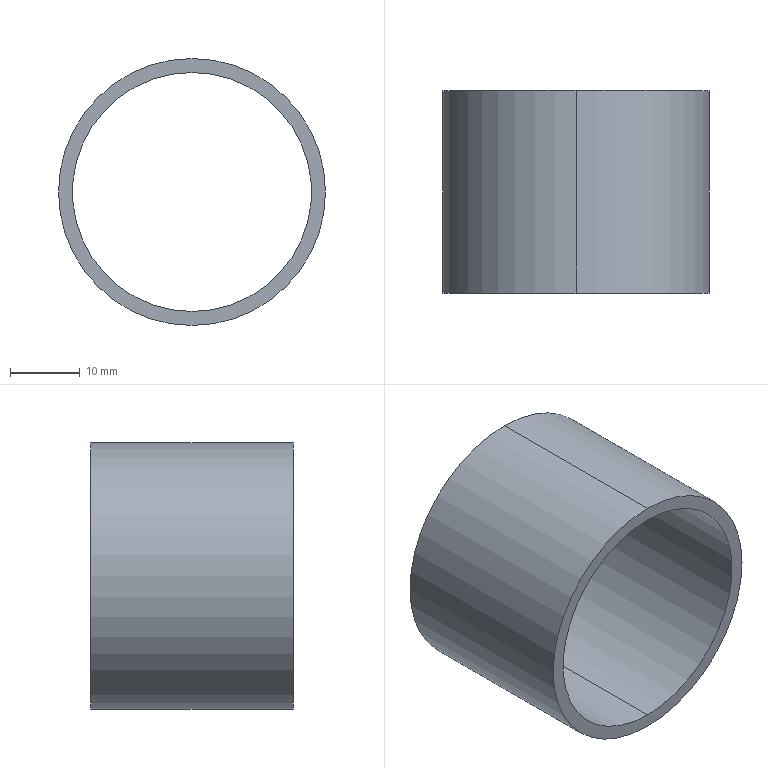Part | STEP file | Middle | 1 solid | 6 faces | box 38.2 x 29 x 38.2 mm | volume 6596 mm3 | cylinder 4 | plane 2 | commonest cylinder face diameters 34.2 x2 38.2 x2
STEP:
#1=CARTESIAN_POINT('',(0.,0.,0.));
#2=DIRECTION('',(0.,0.,1.));
#3=DIRECTION('',(1.,0.,0.));
#4=AXIS2_PLACEMENT_3D('',#1,#2,#3);
#5=CARTESIAN_POINT('',(0.,0.,17.1));
#6=VERTEX_POINT('',#5);
#7=CARTESIAN_POINT('',(0.,29.,17.1));
#8=VERTEX_POINT('',#7);
#9=CARTESIAN_POINT('',(0.,0.,17.1));
#10=DIRECTION('',(0.,1.,0.));
#11=VECTOR('',#10,1.);
#12=LINE('',#9,#11);
#13=CARTESIAN_POINT('',(0.,0.,0.));
#14=DIRECTION('',(0.,1.,0.));
#15=DIRECTION('',(0.,0.,1.));
#16=AXIS2_PLACEMENT_3D('',#13,#14,#15);
#17=CYLINDRICAL_SURFACE('',#16,17.1);
#18=CARTESIAN_POINT('',(6.283,0.));
#19=DIRECTION('',(0.,1.));
#20=VECTOR('',#19,1.);
#21=LINE('',#18,#20);
#22=(GEOMETRIC_REPRESENTATION_CONTEXT(2)PARAMETRIC_REPRESENTATION_CONTEXT()REPRESENTATION_CONTEXT('',''));
#23=DEFINITIONAL_REPRESENTATION('',(#21),#22);
#24=PCURVE('',#17,#23);
#25=CARTESIAN_POINT('',(0.,0.,0.));
#26=DIRECTION('',(0.,1.,0.));
#27=DIRECTION('',(0.,0.,1.));
#28=AXIS2_PLACEMENT_3D('',#25,#26,#27);
#29=CYLINDRICAL_SURFACE('',#28,17.1);
#30=CARTESIAN_POINT('',(0.,0.));
#31=DIRECTION('',(0.,1.));
#32=VECTOR('',#31,1.);
#33=LINE('',#30,#32);
#34=(GEOMETRIC_REPRESENTATION_CONTEXT(2)PARAMETRIC_REPRESENTATION_CONTEXT()REPRESENTATION_CONTEXT('',''));
#35=DEFINITIONAL_REPRESENTATION('',(#33),#34);
#36=PCURVE('',#29,#35);
#37=SURFACE_CURVE('',#12,(#24,#36),.PCURVE_S1.);
#38=EDGE_CURVE('',#6,#8,#37,.T.);
#39=ORIENTED_EDGE('',*,*,#38,.T.);
#40=CARTESIAN_POINT('',(0.,29.,-17.1));
#41=VERTEX_POINT('',#40);
#42=CARTESIAN_POINT('',(0.,29.,0.));
#43=DIRECTION('',(0.,1.,0.));
#44=DIRECTION('',(0.,0.,1.));
#45=AXIS2_PLACEMENT_3D('',#42,#43,#44);
#46=CIRCLE('',#45,17.1);
#47=CARTESIAN_POINT('',(0.,29.));
#48=DIRECTION('',(1.,0.));
#49=VECTOR('',#48,1.);
#50=LINE('',#47,#49);
#51=(GEOMETRIC_REPRESENTATION_CONTEXT(2)PARAMETRIC_REPRESENTATION_CONTEXT()REPRESENTATION_CONTEXT('',''));
#52=DEFINITIONAL_REPRESENTATION('',(#50),#51);
#53=PCURVE('',#17,#52);
#54=CARTESIAN_POINT('',(0.,29.,0.));
#55=DIRECTION('',(0.,1.,0.));
#56=DIRECTION('',(0.,0.,1.));
#57=AXIS2_PLACEMENT_3D('',#54,#55,#56);
#58=PLANE('',#57);
#59=CARTESIAN_POINT('',(0.,0.));
#60=DIRECTION('',(1.,0.));
#61=AXIS2_PLACEMENT_2D('',#59,#60);
#62=CIRCLE('',#61,17.1);
#63=(GEOMETRIC_REPRESENTATION_CONTEXT(2)PARAMETRIC_REPRESENTATION_CONTEXT()REPRESENTATION_CONTEXT('',''));
#64=DEFINITIONAL_REPRESENTATION('',(#62),#63);
#65=PCURVE('',#58,#64);
#66=SURFACE_CURVE('',#46,(#53,#65),.PCURVE_S1.);
#67=EDGE_CURVE('',#41,#8,#66,.T.);
#68=ORIENTED_EDGE('',*,*,#67,.F.);
#69=CARTESIAN_POINT('',(0.,0.,-17.1));
#70=VERTEX_POINT('',#69);
#71=CARTESIAN_POINT('',(0.,0.,-17.1));
#72=DIRECTION('',(0.,1.,0.));
#73=VECTOR('',#72,1.);
#74=LINE('',#71,#73);
#75=CARTESIAN_POINT('',(3.142,0.));
#76=DIRECTION('',(0.,1.));
#77=VECTOR('',#76,1.);
#78=LINE('',#75,#77);
#79=(GEOMETRIC_REPRESENTATION_CONTEXT(2)PARAMETRIC_REPRESENTATION_CONTEXT()REPRESENTATION_CONTEXT('',''));
#80=DEFINITIONAL_REPRESENTATION('',(#78),#79);
#81=PCURVE('',#17,#80);
#82=CARTESIAN_POINT('',(3.142,0.));
#83=DIRECTION('',(0.,1.));
#84=VECTOR('',#83,1.);
#85=LINE('',#82,#84);
#86=(GEOMETRIC_REPRESENTATION_CONTEXT(2)PARAMETRIC_REPRESENTATION_CONTEXT()REPRESENTATION_CONTEXT('',''));
#87=DEFINITIONAL_REPRESENTATION('',(#85),#86);
#88=PCURVE('',#29,#87);
#89=SURFACE_CURVE('',#74,(#81,#88),.PCURVE_S1.);
#90=EDGE_CURVE('',#70,#41,#89,.T.);
#91=ORIENTED_EDGE('',*,*,#90,.F.);
#92=CARTESIAN_POINT('',(0.,0.,0.));
#93=DIRECTION('',(0.,1.,0.));
#94=DIRECTION('',(0.,0.,1.));
#95=AXIS2_PLACEMENT_3D('',#92,#93,#94);
#96=CIRCLE('',#95,17.1);
#97=CARTESIAN_POINT('',(0.,0.));
#98=DIRECTION('',(1.,0.));
#99=VECTOR('',#98,1.);
#100=LINE('',#97,#99);
#101=(GEOMETRIC_REPRESENTATION_CONTEXT(2)PARAMETRIC_REPRESENTATION_CONTEXT()REPRESENTATION_CONTEXT('',''));
#102=DEFINITIONAL_REPRESENTATION('',(#100),#101);
#103=PCURVE('',#17,#102);
#104=CARTESIAN_POINT('',(0.,0.,0.));
#105=DIRECTION('',(0.,1.,0.));
#106=DIRECTION('',(0.,0.,1.));
#107=AXIS2_PLACEMENT_3D('',#104,#105,#106);
#108=PLANE('',#107);
#109=CARTESIAN_POINT('',(0.,0.));
#110=DIRECTION('',(1.,0.));
#111=AXIS2_PLACEMENT_2D('',#109,#110);
#112=CIRCLE('',#111,17.1);
#113=(GEOMETRIC_REPRESENTATION_CONTEXT(2)PARAMETRIC_REPRESENTATION_CONTEXT()REPRESENTATION_CONTEXT('',''));
#114=DEFINITIONAL_REPRESENTATION('',(#112),#113);
#115=PCURVE('',#108,#114);
#116=SURFACE_CURVE('',#96,(#103,#115),.PCURVE_S1.);
#117=EDGE_CURVE('',#70,#6,#116,.T.);
#118=ORIENTED_EDGE('',*,*,#117,.T.);
#119=EDGE_LOOP('',(#39,#68,#91,#118));
#120=FACE_BOUND('',#119,.F.);
#121=ADVANCED_FACE('',(#120),#17,.F.);
#122=CARTESIAN_POINT('',(0.,29.,19.1));
#123=VERTEX_POINT('',#122);
#124=CARTESIAN_POINT('',(0.,29.,-19.1));
#125=VERTEX_POINT('',#124);
#126=CARTESIAN_POINT('',(0.,29.,0.));
#127=DIRECTION('',(0.,1.,0.));
#128=DIRECTION('',(0.,0.,1.));
#129=AXIS2_PLACEMENT_3D('',#126,#127,#128);
#130=CIRCLE('',#129,19.1);
#131=CARTESIAN_POINT('',(0.,29.,0.));
#132=DIRECTION('',(0.,-1.,0.));
#133=DIRECTION('',(0.,0.,-1.));
#134=AXIS2_PLACEMENT_3D('',#131,#132,#133);
#135=CYLINDRICAL_SURFACE('',#134,19.1);
#136=CARTESIAN_POINT('',(3.142,0.));
#137=DIRECTION('',(-1.,0.));
#138=VECTOR('',#137,1.);
#139=LINE('',#136,#138);
#140=(GEOMETRIC_REPRESENTATION_CONTEXT(2)PARAMETRIC_REPRESENTATION_CONTEXT()REPRESENTATION_CONTEXT('',''));
#141=DEFINITIONAL_REPRESENTATION('',(#139),#140);
#142=PCURVE('',#135,#141);
#143=CARTESIAN_POINT('',(0.,0.));
#144=DIRECTION('',(1.,0.));
#145=AXIS2_PLACEMENT_2D('',#143,#144);
#146=CIRCLE('',#145,19.1);
#147=(GEOMETRIC_REPRESENTATION_CONTEXT(2)PARAMETRIC_REPRESENTATION_CONTEXT()REPRESENTATION_CONTEXT('',''));
#148=DEFINITIONAL_REPRESENTATION('',(#146),#147);
#149=PCURVE('',#58,#148);
#150=SURFACE_CURVE('',#130,(#142,#149),.PCURVE_S1.);
#151=EDGE_CURVE('',#123,#125,#150,.T.);
#152=ORIENTED_EDGE('',*,*,#151,.F.);
#153=CARTESIAN_POINT('',(0.,0.,19.1));
#154=VERTEX_POINT('',#153);
#155=CARTESIAN_POINT('',(0.,29.,19.1));
#156=DIRECTION('',(0.,-1.,0.));
#157=VECTOR('',#156,1.);
#158=LINE('',#155,#157);
#159=CARTESIAN_POINT('',(3.142,0.));
#160=DIRECTION('',(0.,1.));
#161=VECTOR('',#160,1.);
#162=LINE('',#159,#161);
#163=(GEOMETRIC_REPRESENTATION_CONTEXT(2)PARAMETRIC_REPRESENTATION_CONTEXT()REPRESENTATION_CONTEXT('',''));
#164=DEFINITIONAL_REPRESENTATION('',(#162),#163);
#165=PCURVE('',#135,#164);
#166=CARTESIAN_POINT('',(0.,29.,0.));
#167=DIRECTION('',(0.,-1.,0.));
#168=DIRECTION('',(0.,0.,-1.));
#169=AXIS2_PLACEMENT_3D('',#166,#167,#168);
#170=CYLINDRICAL_SURFACE('',#169,19.1);
#171=CARTESIAN_POINT('',(3.142,0.));
#172=DIRECTION('',(0.,1.));
#173=VECTOR('',#172,1.);
#174=LINE('',#171,#173);
#175=(GEOMETRIC_REPRESENTATION_CONTEXT(2)PARAMETRIC_REPRESENTATION_CONTEXT()REPRESENTATION_CONTEXT('',''));
#176=DEFINITIONAL_REPRESENTATION('',(#174),#175);
#177=PCURVE('',#170,#176);
#178=SURFACE_CURVE('',#158,(#165,#177),.PCURVE_S1.);
#179=EDGE_CURVE('',#123,#154,#178,.T.);
#180=ORIENTED_EDGE('',*,*,#179,.T.);
#181=CARTESIAN_POINT('',(0.,0.,-19.1));
#182=VERTEX_POINT('',#181);
#183=CARTESIAN_POINT('',(0.,0.,0.));
#184=DIRECTION('',(0.,1.,0.));
#185=DIRECTION('',(0.,0.,1.));
#186=AXIS2_PLACEMENT_3D('',#183,#184,#185);
#187=CIRCLE('',#186,19.1);
#188=CARTESIAN_POINT('',(3.142,29.));
#189=DIRECTION('',(-1.,0.));
#190=VECTOR('',#189,1.);
#191=LINE('',#188,#190);
#192=(GEOMETRIC_REPRESENTATION_CONTEXT(2)PARAMETRIC_REPRESENTATION_CONTEXT()REPRESENTATION_CONTEXT('',''));
#193=DEFINITIONAL_REPRESENTATION('',(#191),#192);
#194=PCURVE('',#135,#193);
#195=CARTESIAN_POINT('',(0.,0.));
#196=DIRECTION('',(1.,0.));
#197=AXIS2_PLACEMENT_2D('',#195,#196);
#198=CIRCLE('',#197,19.1);
#199=(GEOMETRIC_REPRESENTATION_CONTEXT(2)PARAMETRIC_REPRESENTATION_CONTEXT()REPRESENTATION_CONTEXT('',''));
#200=DEFINITIONAL_REPRESENTATION('',(#198),#199);
#201=PCURVE('',#108,#200);
#202=SURFACE_CURVE('',#187,(#194,#201),.PCURVE_S1.);
#203=EDGE_CURVE('',#154,#182,#202,.T.);
#204=ORIENTED_EDGE('',*,*,#203,.T.);
#205=CARTESIAN_POINT('',(0.,29.,-19.1));
#206=DIRECTION('',(0.,-1.,0.));
#207=VECTOR('',#206,1.);
#208=LINE('',#205,#207);
#209=CARTESIAN_POINT('',(0.,0.));
#210=DIRECTION('',(0.,1.));
#211=VECTOR('',#210,1.);
#212=LINE('',#209,#211);
#213=(GEOMETRIC_REPRESENTATION_CONTEXT(2)PARAMETRIC_REPRESENTATION_CONTEXT()REPRESENTATION_CONTEXT('',''));
#214=DEFINITIONAL_REPRESENTATION('',(#212),#213);
#215=PCURVE('',#135,#214);
#216=CARTESIAN_POINT('',(6.283,0.));
#217=DIRECTION('',(0.,1.));
#218=VECTOR('',#217,1.);
#219=LINE('',#216,#218);
#220=(GEOMETRIC_REPRESENTATION_CONTEXT(2)PARAMETRIC_REPRESENTATION_CONTEXT()REPRESENTATION_CONTEXT('',''));
#221=DEFINITIONAL_REPRESENTATION('',(#219),#220);
#222=PCURVE('',#170,#221);
#223=SURFACE_CURVE('',#208,(#215,#222),.PCURVE_S1.);
#224=EDGE_CURVE('',#125,#182,#223,.T.);
#225=ORIENTED_EDGE('',*,*,#224,.F.);
#226=EDGE_LOOP('',(#152,#180,#204,#225));
#227=FACE_BOUND('',#226,.T.);
#228=ADVANCED_FACE('',(#227),#135,.T.);
#229=ORIENTED_EDGE('',*,*,#179,.F.);
#230=CARTESIAN_POINT('',(0.,29.,0.));
#231=DIRECTION('',(0.,1.,0.));
#232=DIRECTION('',(0.,0.,1.));
#233=AXIS2_PLACEMENT_3D('',#230,#231,#232);
#234=CIRCLE('',#233,19.1);
#235=CARTESIAN_POINT('',(9.425,0.));
#236=DIRECTION('',(-1.,0.));
#237=VECTOR('',#236,1.);
#238=LINE('',#235,#237);
#239=(GEOMETRIC_REPRESENTATION_CONTEXT(2)PARAMETRIC_REPRESENTATION_CONTEXT()REPRESENTATION_CONTEXT('',''));
#240=DEFINITIONAL_REPRESENTATION('',(#238),#239);
#241=PCURVE('',#170,#240);
#242=CARTESIAN_POINT('',(0.,0.));
#243=DIRECTION('',(1.,0.));
#244=AXIS2_PLACEMENT_2D('',#242,#243);
#245=CIRCLE('',#244,19.1);
#246=(GEOMETRIC_REPRESENTATION_CONTEXT(2)PARAMETRIC_REPRESENTATION_CONTEXT()REPRESENTATION_CONTEXT('',''));
#247=DEFINITIONAL_REPRESENTATION('',(#245),#246);
#248=PCURVE('',#58,#247);
#249=SURFACE_CURVE('',#234,(#241,#248),.PCURVE_S1.);
#250=EDGE_CURVE('',#125,#123,#249,.T.);
#251=ORIENTED_EDGE('',*,*,#250,.F.);
#252=ORIENTED_EDGE('',*,*,#224,.T.);
#253=CARTESIAN_POINT('',(0.,0.,0.));
#254=DIRECTION('',(0.,1.,0.));
#255=DIRECTION('',(0.,0.,1.));
#256=AXIS2_PLACEMENT_3D('',#253,#254,#255);
#257=CIRCLE('',#256,19.1);
#258=CARTESIAN_POINT('',(9.425,29.));
#259=DIRECTION('',(-1.,0.));
#260=VECTOR('',#259,1.);
#261=LINE('',#258,#260);
#262=(GEOMETRIC_REPRESENTATION_CONTEXT(2)PARAMETRIC_REPRESENTATION_CONTEXT()REPRESENTATION_CONTEXT('',''));
#263=DEFINITIONAL_REPRESENTATION('',(#261),#262);
#264=PCURVE('',#170,#263);
#265=CARTESIAN_POINT('',(0.,0.));
#266=DIRECTION('',(1.,0.));
#267=AXIS2_PLACEMENT_2D('',#265,#266);
#268=CIRCLE('',#267,19.1);
#269=(GEOMETRIC_REPRESENTATION_CONTEXT(2)PARAMETRIC_REPRESENTATION_CONTEXT()REPRESENTATION_CONTEXT('',''));
#270=DEFINITIONAL_REPRESENTATION('',(#268),#269);
#271=PCURVE('',#108,#270);
#272=SURFACE_CURVE('',#257,(#264,#271),.PCURVE_S1.);
#273=EDGE_CURVE('',#182,#154,#272,.T.);
#274=ORIENTED_EDGE('',*,*,#273,.T.);
#275=EDGE_LOOP('',(#229,#251,#252,#274));
#276=FACE_BOUND('',#275,.T.);
#277=ADVANCED_FACE('',(#276),#170,.T.);
#278=CARTESIAN_POINT('',(0.,29.,0.));
#279=DIRECTION('',(0.,1.,0.));
#280=DIRECTION('',(0.,0.,1.));
#281=AXIS2_PLACEMENT_3D('',#278,#279,#280);
#282=CIRCLE('',#281,17.1);
#283=CARTESIAN_POINT('',(0.,0.));
#284=DIRECTION('',(1.,0.));
#285=AXIS2_PLACEMENT_2D('',#283,#284);
#286=CIRCLE('',#285,17.1);
#287=(GEOMETRIC_REPRESENTATION_CONTEXT(2)PARAMETRIC_REPRESENTATION_CONTEXT()REPRESENTATION_CONTEXT('',''));
#288=DEFINITIONAL_REPRESENTATION('',(#286),#287);
#289=PCURVE('',#58,#288);
#290=CARTESIAN_POINT('',(0.,29.));
#291=DIRECTION('',(1.,0.));
#292=VECTOR('',#291,1.);
#293=LINE('',#290,#292);
#294=(GEOMETRIC_REPRESENTATION_CONTEXT(2)PARAMETRIC_REPRESENTATION_CONTEXT()REPRESENTATION_CONTEXT('',''));
#295=DEFINITIONAL_REPRESENTATION('',(#293),#294);
#296=PCURVE('',#29,#295);
#297=SURFACE_CURVE('',#282,(#289,#296),.PCURVE_S1.);
#298=EDGE_CURVE('',#8,#41,#297,.T.);
#299=ORIENTED_EDGE('',*,*,#298,.F.);
#300=ORIENTED_EDGE('',*,*,#67,.F.);
#301=EDGE_LOOP('',(#299,#300));
#302=FACE_BOUND('',#301,.T.);
#303=ORIENTED_EDGE('',*,*,#250,.T.);
#304=ORIENTED_EDGE('',*,*,#151,.T.);
#305=EDGE_LOOP('',(#303,#304));
#306=FACE_BOUND('',#305,.T.);
#307=ADVANCED_FACE('',(#302,#306),#58,.T.);
#308=CARTESIAN_POINT('',(0.,0.,0.));
#309=DIRECTION('',(0.,1.,0.));
#310=DIRECTION('',(0.,0.,1.));
#311=AXIS2_PLACEMENT_3D('',#308,#309,#310);
#312=CIRCLE('',#311,17.1);
#313=CARTESIAN_POINT('',(0.,0.));
#314=DIRECTION('',(1.,0.));
#315=AXIS2_PLACEMENT_2D('',#313,#314);
#316=CIRCLE('',#315,17.1);
#317=(GEOMETRIC_REPRESENTATION_CONTEXT(2)PARAMETRIC_REPRESENTATION_CONTEXT()REPRESENTATION_CONTEXT('',''));
#318=DEFINITIONAL_REPRESENTATION('',(#316),#317);
#319=PCURVE('',#108,#318);
#320=CARTESIAN_POINT('',(0.,0.));
#321=DIRECTION('',(1.,0.));
#322=VECTOR('',#321,1.);
#323=LINE('',#320,#322);
#324=(GEOMETRIC_REPRESENTATION_CONTEXT(2)PARAMETRIC_REPRESENTATION_CONTEXT()REPRESENTATION_CONTEXT('',''));
#325=DEFINITIONAL_REPRESENTATION('',(#323),#324);
#326=PCURVE('',#29,#325);
#327=SURFACE_CURVE('',#312,(#319,#326),.PCURVE_S1.);
#328=EDGE_CURVE('',#6,#70,#327,.T.);
#329=ORIENTED_EDGE('',*,*,#328,.T.);
#330=ORIENTED_EDGE('',*,*,#117,.T.);
#331=EDGE_LOOP('',(#329,#330));
#332=FACE_BOUND('',#331,.T.);
#333=ORIENTED_EDGE('',*,*,#273,.F.);
#334=ORIENTED_EDGE('',*,*,#203,.F.);
#335=EDGE_LOOP('',(#333,#334));
#336=FACE_BOUND('',#335,.T.);
#337=ADVANCED_FACE('',(#332,#336),#108,.F.);
#338=ORIENTED_EDGE('',*,*,#298,.F.);
#339=ORIENTED_EDGE('',*,*,#38,.F.);
#340=ORIENTED_EDGE('',*,*,#328,.T.);
#341=ORIENTED_EDGE('',*,*,#90,.T.);
#342=EDGE_LOOP('',(#338,#339,#340,#341));
#343=FACE_BOUND('',#342,.F.);
#344=ADVANCED_FACE('',(#343),#29,.F.);
#345=CLOSED_SHELL('',(#121,#228,#277,#307,#337,#344));
#346=MANIFOLD_SOLID_BREP('',#345);
#347=(LENGTH_UNIT()NAMED_UNIT(*)SI_UNIT(.MILLI.,.METRE.));
#348=UNCERTAINTY_MEASURE_WITH_UNIT(LENGTH_MEASURE(0.0000001),#347,'','');
#349=(NAMED_UNIT(*)PLANE_ANGLE_UNIT()SI_UNIT($,.RADIAN.));
#350=(NAMED_UNIT(*)SI_UNIT($,.STERADIAN.)SOLID_ANGLE_UNIT());
#351=(GEOMETRIC_REPRESENTATION_CONTEXT(3)GLOBAL_UNCERTAINTY_ASSIGNED_CONTEXT((#348))GLOBAL_UNIT_ASSIGNED_CONTEXT((#347,#349,#350))REPRESENTATION_CONTEXT('',''));
#352=ADVANCED_BREP_SHAPE_REPRESENTATION('',(#4,#346),#351);